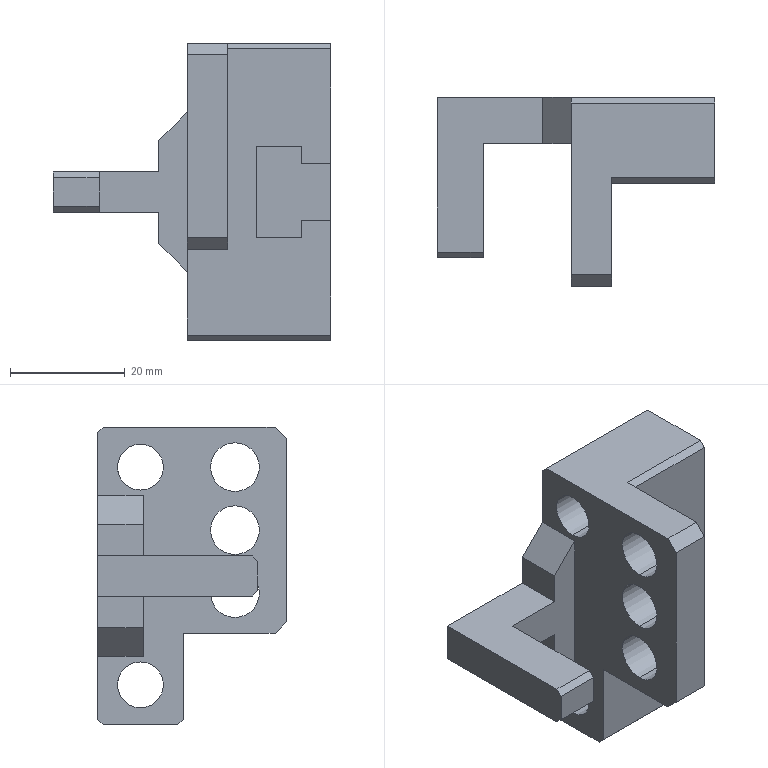Part | STEP file | discharge block | 2 solids | 65 faces | box 48.4 x 33 x 52 mm | volume 23054 mm3 | plane 45 | cylinder 18 | cone 2 | commonest cylinder face diameters 8.5 x6 3.3 x4 4.2 x4 8 x4